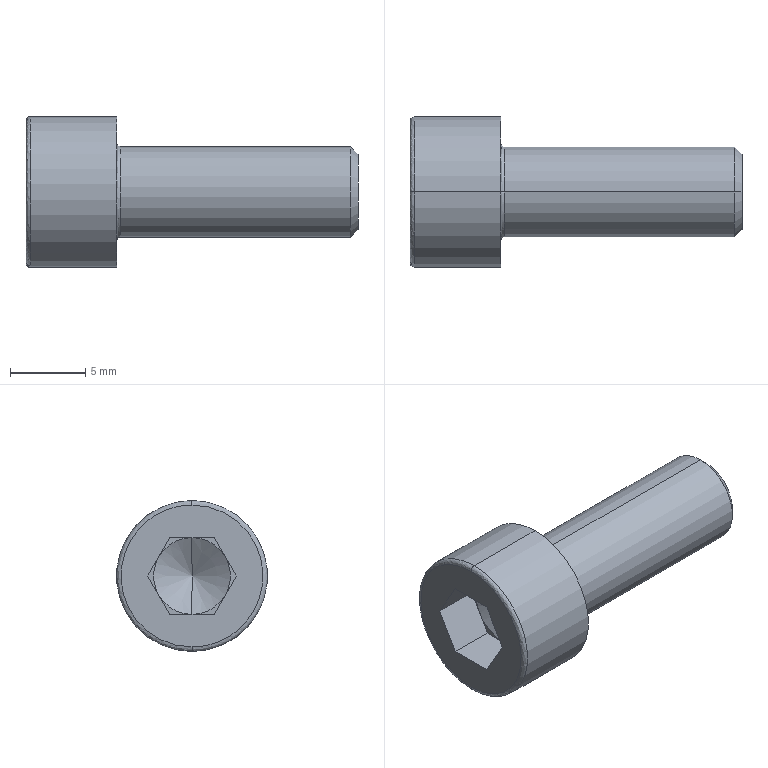Part | STEP file | PN_0066_default | 1 solid | 27 faces | box 22 x 10 x 10 mm | volume 844.002 mm3 | plane 15 | spline 4 | cone 4 | cylinder 4 | commonest cylinder face diameters 6 x2 10 x2